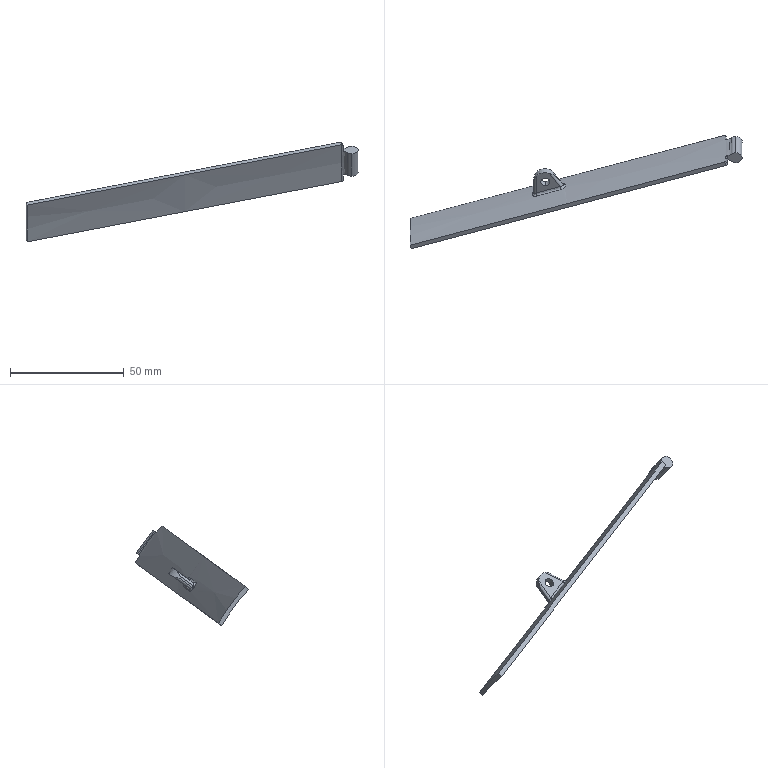Part | STEP file | Completa.sldasm-Part-149_Valor predeterminado | 1 solid | 38 faces | box 146.027 x 49.831 x 43.834 mm | volume 6463 mm3 | cylinder 15 | plane 10 | spline 9 | cone 3 | torus 1 | commonest cylinder face diameters 1 x5 2 x4 5.5 x3 4 x2 10 x1